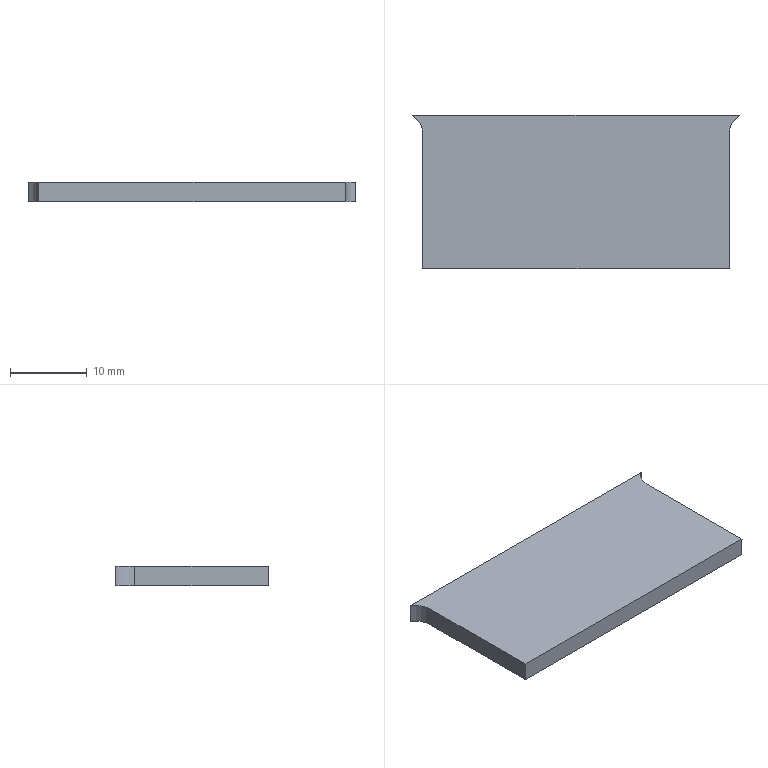Part | STEP file | lll_id990_x_t | 1 solid | 8 faces | box 42.684 x 20 x 2.5 mm | volume 2005 mm3 | plane 6 | cylinder 2 | commonest cylinder face diameters 6 x2
STEP:
#1=CARTESIAN_POINT('',(2991.342,40.5,2.5));
#2=VERTEX_POINT('',#1);
#3=CARTESIAN_POINT('',(2991.342,40.5,-0.000000212));
#4=VERTEX_POINT('',#3);
#5=CARTESIAN_POINT('',(2991.342,40.5,1.25));
#6=DIRECTION('',(0.000000011,0.000000008,-1.));
#7=VECTOR('',#6,1.);
#8=LINE('',#5,#7);
#9=EDGE_CURVE('',#2,#4,#8,.T.);
#10=ORIENTED_EDGE('',*,*,#9,.T.);
#11=CARTESIAN_POINT('',(2948.658,40.5,0.));
#12=VERTEX_POINT('',#11);
#13=CARTESIAN_POINT('',(13471.883,40.5,0.));
#14=DIRECTION('',(-1.,0.,0.));
#15=VECTOR('',#14,1.);
#16=LINE('',#13,#15);
#17=EDGE_CURVE('',#4,#12,#16,.T.);
#18=ORIENTED_EDGE('',*,*,#17,.T.);
#19=CARTESIAN_POINT('',(2948.658,40.5,2.5));
#20=VERTEX_POINT('',#19);
#21=CARTESIAN_POINT('',(2948.658,40.5,1.25));
#22=DIRECTION('',(-0.000000011,0.000000008,-1.));
#23=VECTOR('',#22,1.);
#24=LINE('',#21,#23);
#25=EDGE_CURVE('',#20,#12,#24,.T.);
#26=ORIENTED_EDGE('',*,*,#25,.F.);
#27=CARTESIAN_POINT('',(13471.883,40.5,2.5));
#28=DIRECTION('',(1.,0.,0.));
#29=VECTOR('',#28,1.);
#30=LINE('',#27,#29);
#31=EDGE_CURVE('',#20,#2,#30,.T.);
#32=ORIENTED_EDGE('',*,*,#31,.T.);
#33=EDGE_LOOP('',(#10,#18,#26,#32));
#34=FACE_OUTER_BOUND('',#33,.T.);
#35=CARTESIAN_POINT('',(2930.426,40.5,2.5));
#36=DIRECTION('',(0.,-1.,-0.000000008));
#37=DIRECTION('',(0.,-0.000000008,1.));
#38=AXIS2_PLACEMENT_3D('',#35,#36,#37);
#39=PLANE('',#38);
#40=ADVANCED_FACE('',(#34),#39,.F.);
#41=ORIENTED_EDGE('',*,*,#9,.F.);
#42=CARTESIAN_POINT('',(2990.,38.,2.5));
#43=VERTEX_POINT('',#42);
#44=CARTESIAN_POINT('',(2993.,38.,2.5));
#45=DIRECTION('',(0.,0.,1.));
#46=DIRECTION('',(-1.,0.,0.));
#47=AXIS2_PLACEMENT_3D('',#44,#45,#46);
#48=CIRCLE('',#47,3.);
#49=EDGE_CURVE('',#2,#43,#48,.T.);
#50=ORIENTED_EDGE('',*,*,#49,.T.);
#51=CARTESIAN_POINT('',(2990.,38.,0.));
#52=VERTEX_POINT('',#51);
#53=CARTESIAN_POINT('',(2990.,38.,2.5));
#54=DIRECTION('',(0.,0.,1.));
#55=VECTOR('',#54,1.);
#56=LINE('',#53,#55);
#57=EDGE_CURVE('',#52,#43,#56,.T.);
#58=ORIENTED_EDGE('',*,*,#57,.F.);
#59=CARTESIAN_POINT('',(2993.,38.,0.));
#60=DIRECTION('',(0.,0.,1.));
#61=DIRECTION('',(-1.,0.,0.));
#62=AXIS2_PLACEMENT_3D('',#59,#60,#61);
#63=CIRCLE('',#62,3.);
#64=EDGE_CURVE('',#4,#52,#63,.T.);
#65=ORIENTED_EDGE('',*,*,#64,.F.);
#66=EDGE_LOOP('',(#41,#50,#58,#65));
#67=FACE_OUTER_BOUND('',#66,.T.);
#68=CARTESIAN_POINT('',(2993.,38.,2.5));
#69=DIRECTION('',(0.,0.,-1.));
#70=DIRECTION('',(-1.,0.,0.));
#71=AXIS2_PLACEMENT_3D('',#68,#69,#70);
#72=CYLINDRICAL_SURFACE('',#71,3.);
#73=ADVANCED_FACE('',(#67),#72,.F.);
#74=CARTESIAN_POINT('',(2950.,38.,2.5));
#75=VERTEX_POINT('',#74);
#76=CARTESIAN_POINT('',(2947.,38.,2.5));
#77=DIRECTION('',(0.,0.,-1.));
#78=DIRECTION('',(-1.,0.,0.));
#79=AXIS2_PLACEMENT_3D('',#76,#77,#78);
#80=CIRCLE('',#79,3.);
#81=EDGE_CURVE('',#20,#75,#80,.T.);
#82=ORIENTED_EDGE('',*,*,#81,.F.);
#83=ORIENTED_EDGE('',*,*,#25,.T.);
#84=CARTESIAN_POINT('',(2950.,38.,0.));
#85=VERTEX_POINT('',#84);
#86=CARTESIAN_POINT('',(2947.,38.,0.));
#87=DIRECTION('',(0.,0.,-1.));
#88=DIRECTION('',(-1.,0.,0.));
#89=AXIS2_PLACEMENT_3D('',#86,#87,#88);
#90=CIRCLE('',#89,3.);
#91=EDGE_CURVE('',#12,#85,#90,.T.);
#92=ORIENTED_EDGE('',*,*,#91,.T.);
#93=CARTESIAN_POINT('',(2950.,38.,2.5));
#94=DIRECTION('',(0.,0.,1.));
#95=VECTOR('',#94,1.);
#96=LINE('',#93,#95);
#97=EDGE_CURVE('',#85,#75,#96,.T.);
#98=ORIENTED_EDGE('',*,*,#97,.T.);
#99=EDGE_LOOP('',(#82,#83,#92,#98));
#100=FACE_OUTER_BOUND('',#99,.T.);
#101=CARTESIAN_POINT('',(2947.,38.,2.5));
#102=DIRECTION('',(0.,0.,-1.));
#103=DIRECTION('',(-1.,0.,0.));
#104=AXIS2_PLACEMENT_3D('',#101,#102,#103);
#105=CYLINDRICAL_SURFACE('',#104,3.);
#106=ADVANCED_FACE('',(#100),#105,.F.);
#107=CARTESIAN_POINT('',(2990.,20.5,2.5));
#108=VERTEX_POINT('',#107);
#109=CARTESIAN_POINT('',(2990.,20.5,0.));
#110=VERTEX_POINT('',#109);
#111=CARTESIAN_POINT('',(2990.,20.5,2.5));
#112=DIRECTION('',(0.,0.000000008,-1.));
#113=VECTOR('',#112,1.);
#114=LINE('',#111,#113);
#115=EDGE_CURVE('',#108,#110,#114,.T.);
#116=ORIENTED_EDGE('',*,*,#115,.T.);
#117=CARTESIAN_POINT('',(2990.,38.,0.));
#118=DIRECTION('',(0.,-1.,0.));
#119=VECTOR('',#118,1.);
#120=LINE('',#117,#119);
#121=EDGE_CURVE('',#52,#110,#120,.T.);
#122=ORIENTED_EDGE('',*,*,#121,.F.);
#123=ORIENTED_EDGE('',*,*,#57,.T.);
#124=CARTESIAN_POINT('',(2990.,38.,2.5));
#125=DIRECTION('',(0.,-1.,0.));
#126=VECTOR('',#125,1.);
#127=LINE('',#124,#126);
#128=EDGE_CURVE('',#43,#108,#127,.T.);
#129=ORIENTED_EDGE('',*,*,#128,.T.);
#130=EDGE_LOOP('',(#116,#122,#123,#129));
#131=FACE_OUTER_BOUND('',#130,.T.);
#132=CARTESIAN_POINT('',(2990.,38.,2.5));
#133=DIRECTION('',(1.,0.,0.));
#134=DIRECTION('',(0.,0.,-1.));
#135=AXIS2_PLACEMENT_3D('',#132,#133,#134);
#136=PLANE('',#135);
#137=ADVANCED_FACE('',(#131),#136,.T.);
#138=CARTESIAN_POINT('',(2950.,20.5,0.));
#139=VERTEX_POINT('',#138);
#140=CARTESIAN_POINT('',(2950.,38.,0.));
#141=DIRECTION('',(0.,-1.,0.));
#142=VECTOR('',#141,1.);
#143=LINE('',#140,#142);
#144=EDGE_CURVE('',#85,#139,#143,.T.);
#145=ORIENTED_EDGE('',*,*,#144,.T.);
#146=CARTESIAN_POINT('',(2950.,20.5,2.5));
#147=VERTEX_POINT('',#146);
#148=CARTESIAN_POINT('',(2950.,20.5,2.5));
#149=DIRECTION('',(0.,-0.000000008,1.));
#150=VECTOR('',#149,1.);
#151=LINE('',#148,#150);
#152=EDGE_CURVE('',#139,#147,#151,.T.);
#153=ORIENTED_EDGE('',*,*,#152,.T.);
#154=CARTESIAN_POINT('',(2950.,38.,2.5));
#155=DIRECTION('',(0.,-1.,0.));
#156=VECTOR('',#155,1.);
#157=LINE('',#154,#156);
#158=EDGE_CURVE('',#75,#147,#157,.T.);
#159=ORIENTED_EDGE('',*,*,#158,.F.);
#160=ORIENTED_EDGE('',*,*,#97,.F.);
#161=EDGE_LOOP('',(#145,#153,#159,#160));
#162=FACE_OUTER_BOUND('',#161,.T.);
#163=CARTESIAN_POINT('',(2950.,38.,2.5));
#164=DIRECTION('',(1.,0.,0.));
#165=DIRECTION('',(0.,0.,-1.));
#166=AXIS2_PLACEMENT_3D('',#163,#164,#165);
#167=PLANE('',#166);
#168=ADVANCED_FACE('',(#162),#167,.F.);
#169=ORIENTED_EDGE('',*,*,#158,.T.);
#170=CARTESIAN_POINT('',(13471.883,20.5,2.5));
#171=DIRECTION('',(1.,0.,0.));
#172=VECTOR('',#171,1.);
#173=LINE('',#170,#172);
#174=EDGE_CURVE('',#147,#108,#173,.T.);
#175=ORIENTED_EDGE('',*,*,#174,.T.);
#176=ORIENTED_EDGE('',*,*,#128,.F.);
#177=ORIENTED_EDGE('',*,*,#49,.F.);
#178=ORIENTED_EDGE('',*,*,#31,.F.);
#179=ORIENTED_EDGE('',*,*,#81,.T.);
#180=EDGE_LOOP('',(#169,#175,#176,#177,#178,#179));
#181=FACE_OUTER_BOUND('',#180,.T.);
#182=CARTESIAN_POINT('',(13471.883,-13712.786,2.5));
#183=DIRECTION('',(0.,0.,-1.));
#184=DIRECTION('',(-1.,0.,0.));
#185=AXIS2_PLACEMENT_3D('',#182,#183,#184);
#186=PLANE('',#185);
#187=ADVANCED_FACE('',(#181),#186,.F.);
#188=CARTESIAN_POINT('',(13471.883,20.5,0.));
#189=DIRECTION('',(1.,0.,0.));
#190=VECTOR('',#189,1.);
#191=LINE('',#188,#190);
#192=EDGE_CURVE('',#139,#110,#191,.T.);
#193=ORIENTED_EDGE('',*,*,#192,.F.);
#194=ORIENTED_EDGE('',*,*,#144,.F.);
#195=ORIENTED_EDGE('',*,*,#91,.F.);
#196=ORIENTED_EDGE('',*,*,#17,.F.);
#197=ORIENTED_EDGE('',*,*,#64,.T.);
#198=ORIENTED_EDGE('',*,*,#121,.T.);
#199=EDGE_LOOP('',(#193,#194,#195,#196,#197,#198));
#200=FACE_OUTER_BOUND('',#199,.T.);
#201=CARTESIAN_POINT('',(13471.883,-13712.786,0.));
#202=DIRECTION('',(0.,0.,-1.));
#203=DIRECTION('',(-1.,0.,0.));
#204=AXIS2_PLACEMENT_3D('',#201,#202,#203);
#205=PLANE('',#204);
#206=ADVANCED_FACE('',(#200),#205,.T.);
#207=ORIENTED_EDGE('',*,*,#115,.F.);
#208=ORIENTED_EDGE('',*,*,#174,.F.);
#209=ORIENTED_EDGE('',*,*,#152,.F.);
#210=ORIENTED_EDGE('',*,*,#192,.T.);
#211=EDGE_LOOP('',(#207,#208,#209,#210));
#212=FACE_OUTER_BOUND('',#211,.T.);
#213=CARTESIAN_POINT('',(2970.,20.5,1.25));
#214=DIRECTION('',(0.,1.,0.000000008));
#215=DIRECTION('',(0.,-0.000000008,1.));
#216=AXIS2_PLACEMENT_3D('',#213,#214,#215);
#217=PLANE('',#216);
#218=ADVANCED_FACE('',(#212),#217,.F.);
#219=CLOSED_SHELL('',(#40,#73,#106,#137,#168,#187,#206,#218));
#220=MANIFOLD_SOLID_BREP('',#219);
#221=(LENGTH_UNIT()NAMED_UNIT(*)SI_UNIT(.MILLI.,.METRE.));
#222=UNCERTAINTY_MEASURE_WITH_UNIT(LENGTH_MEASURE(0.00002),#221,'','');
#223=(NAMED_UNIT(*)PLANE_ANGLE_UNIT()SI_UNIT($,.RADIAN.));
#224=PLANE_ANGLE_MEASURE_WITH_UNIT(PLANE_ANGLE_MEASURE(0.01745),#223);
#225=DIMENSIONAL_EXPONENTS(0.,0.,0.,0.,0.,0.,0.);
#226=(CONVERSION_BASED_UNIT('DEGREE',#224)NAMED_UNIT(#225)PLANE_ANGLE_UNIT());
#227=(NAMED_UNIT(*)SI_UNIT($,.STERADIAN.)SOLID_ANGLE_UNIT());
#228=(GEOMETRIC_REPRESENTATION_CONTEXT(3)GLOBAL_UNCERTAINTY_ASSIGNED_CONTEXT((#222))GLOBAL_UNIT_ASSIGNED_CONTEXT((#221,#226,#227))REPRESENTATION_CONTEXT('',''));
#229=ADVANCED_BREP_SHAPE_REPRESENTATION('',(#220),#228);